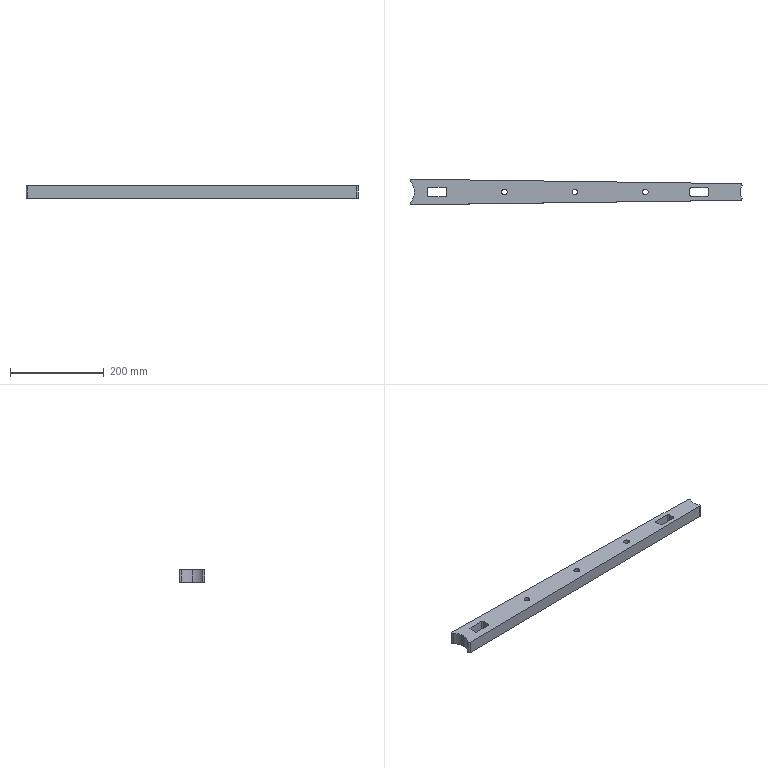Part | STEP file | Belt support QY-1-31 | 1 solid | 35 faces | box 707.006 x 54.439 x 27 mm | volume 797280 mm3 | cylinder 23 | plane 12 | commonest cylinder face diameters 6 x10 12 x6 4 x4 64.521 x2 47.927 x1